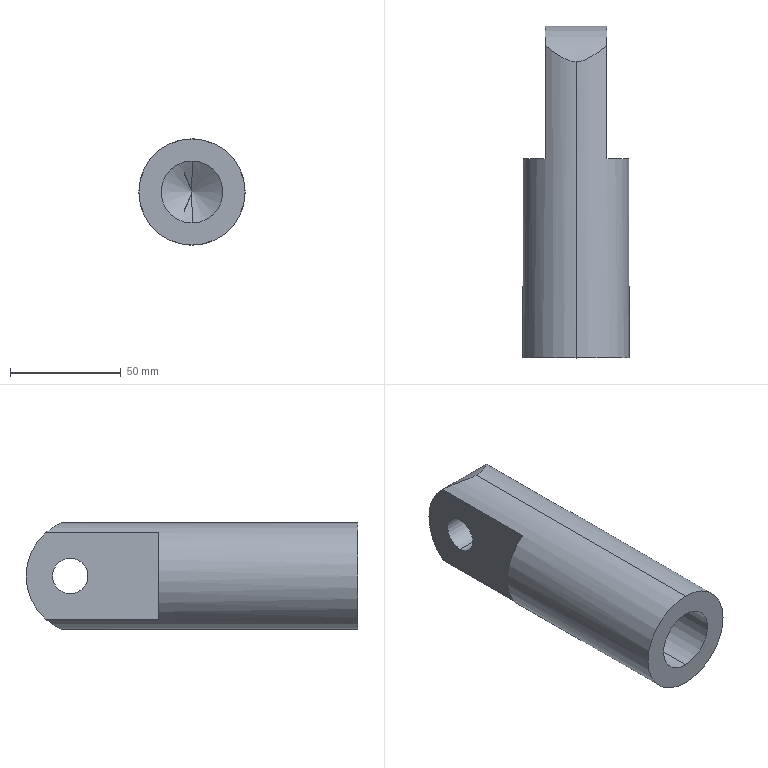Part | STEP file | PN_0021 Connecting shaft | 1 solid | 14 faces | box 48 x 150 x 48 mm | volume 198072 mm3 | cylinder 7 | plane 5 | cone 2 | commonest cylinder face diameters 16 x2 28 x2 48 x2 51.816 x1